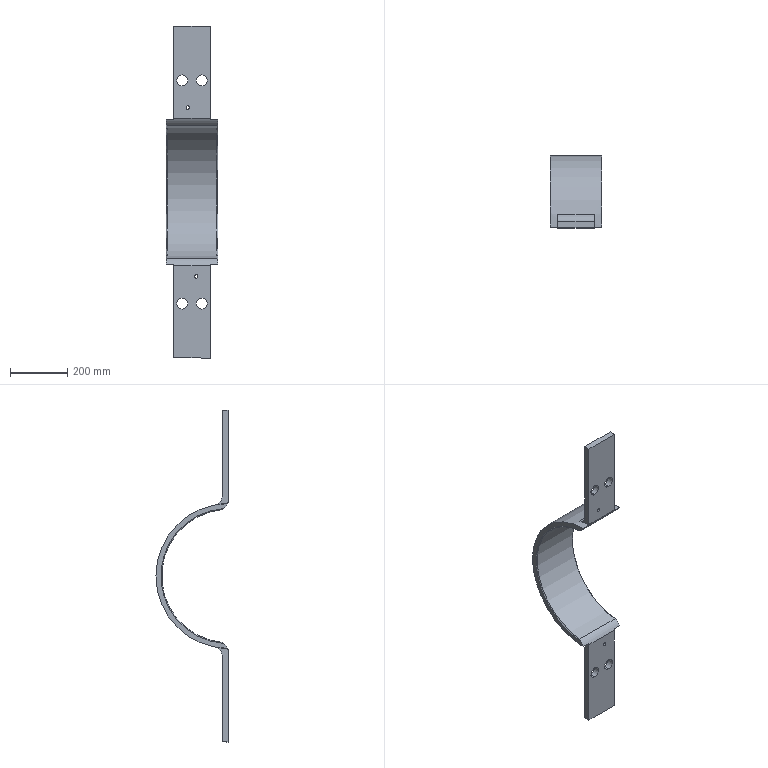Part | SolidWorks | features ICE 4, Fillet 2, MirrorPattern 2, Chamfer 1, Extrusion 1 | 1 solid | 32 faces | box 180 x 251.8 x 1160 mm | volume 4313938 mm3 | cylinder 18 | plane 12 | cone 2 | commonest cylinder face diameters 38 x8 12 x4 60 x2 110 x2 466 x1 506 x1
STEP:
#1=CARTESIAN_POINT('',(15.,22.,-301.));
#2=VERTEX_POINT('',#1);
#3=CARTESIAN_POINT('',(15.,22.,-289.));
#4=VERTEX_POINT('',#3);
#5=CARTESIAN_POINT('',(15.,22.,-295.));
#6=DIRECTION('',(0.,1.,0.));
#7=DIRECTION('',(0.,0.,-1.));
#8=AXIS2_PLACEMENT_3D('',#5,#6,#7);
#9=CIRCLE('',#8,6.);
#10=EDGE_CURVE('',#2,#4,#9,.T.);
#11=ORIENTED_EDGE('',*,*,#10,.T.);
#12=CARTESIAN_POINT('',(15.,1.2,-289.));
#13=VERTEX_POINT('',#12);
#14=CARTESIAN_POINT('',(15.,1.2,-289.));
#15=DIRECTION('',(0.,-1.,0.));
#16=VECTOR('',#15,1000.);
#17=LINE('',#14,#16);
#18=EDGE_CURVE('',#4,#13,#17,.T.);
#19=ORIENTED_EDGE('',*,*,#18,.T.);
#20=CARTESIAN_POINT('',(15.,1.2,-301.));
#21=VERTEX_POINT('',#20);
#22=CARTESIAN_POINT('',(15.,1.2,-295.));
#23=DIRECTION('',(0.,-1.,0.));
#24=DIRECTION('',(0.,0.,1.));
#25=AXIS2_PLACEMENT_3D('',#22,#23,#24);
#26=CIRCLE('',#25,6.);
#27=EDGE_CURVE('',#13,#21,#26,.T.);
#28=ORIENTED_EDGE('',*,*,#27,.T.);
#29=CARTESIAN_POINT('',(15.,1.2,-301.));
#30=DIRECTION('',(0.,-1.,0.));
#31=VECTOR('',#30,1000.);
#32=LINE('',#29,#31);
#33=EDGE_CURVE('',#2,#21,#32,.T.);
#34=ORIENTED_EDGE('',*,*,#33,.F.);
#35=EDGE_LOOP('',(#11,#19,#28,#34));
#36=FACE_OUTER_BOUND('',#35,.T.);
#37=CARTESIAN_POINT('',(15.,1.2,-295.));
#38=DIRECTION('',(0.,-1.,0.));
#39=DIRECTION('',(0.,0.,-1.));
#40=AXIS2_PLACEMENT_3D('',#37,#38,#39);
#41=CYLINDRICAL_SURFACE('',#40,6.);
#42=ADVANCED_FACE('',(#36),#41,.F.);
#43=CARTESIAN_POINT('',(-15.,22.,289.));
#44=VERTEX_POINT('',#43);
#45=CARTESIAN_POINT('',(-15.,22.,301.));
#46=VERTEX_POINT('',#45);
#47=CARTESIAN_POINT('',(-15.,22.,295.));
#48=DIRECTION('',(0.,1.,0.));
#49=DIRECTION('',(0.,0.,-1.));
#50=AXIS2_PLACEMENT_3D('',#47,#48,#49);
#51=CIRCLE('',#50,6.);
#52=EDGE_CURVE('',#44,#46,#51,.T.);
#53=ORIENTED_EDGE('',*,*,#52,.T.);
#54=CARTESIAN_POINT('',(-15.,1.2,301.));
#55=VERTEX_POINT('',#54);
#56=CARTESIAN_POINT('',(-15.,1.2,301.));
#57=DIRECTION('',(0.,-1.,0.));
#58=VECTOR('',#57,1000.);
#59=LINE('',#56,#58);
#60=EDGE_CURVE('',#46,#55,#59,.T.);
#61=ORIENTED_EDGE('',*,*,#60,.T.);
#62=CARTESIAN_POINT('',(-15.,1.2,289.));
#63=VERTEX_POINT('',#62);
#64=CARTESIAN_POINT('',(-15.,1.2,295.));
#65=DIRECTION('',(0.,-1.,0.));
#66=DIRECTION('',(0.,0.,1.));
#67=AXIS2_PLACEMENT_3D('',#64,#65,#66);
#68=CIRCLE('',#67,6.);
#69=EDGE_CURVE('',#55,#63,#68,.T.);
#70=ORIENTED_EDGE('',*,*,#69,.T.);
#71=CARTESIAN_POINT('',(-15.,1.2,289.));
#72=DIRECTION('',(0.,-1.,0.));
#73=VECTOR('',#72,1000.);
#74=LINE('',#71,#73);
#75=EDGE_CURVE('',#44,#63,#74,.T.);
#76=ORIENTED_EDGE('',*,*,#75,.F.);
#77=EDGE_LOOP('',(#53,#61,#70,#76));
#78=FACE_OUTER_BOUND('',#77,.T.);
#79=CARTESIAN_POINT('',(-15.,1.2,295.));
#80=DIRECTION('',(0.,-1.,0.));
#81=DIRECTION('',(0.,0.,-1.));
#82=AXIS2_PLACEMENT_3D('',#79,#80,#81);
#83=CYLINDRICAL_SURFACE('',#82,6.);
#84=ADVANCED_FACE('',(#78),#83,.F.);
#85=CARTESIAN_POINT('',(-34.,22.,-409.));
#86=VERTEX_POINT('',#85);
#87=CARTESIAN_POINT('',(-34.,22.,-371.));
#88=VERTEX_POINT('',#87);
#89=CARTESIAN_POINT('',(-34.,22.,-390.));
#90=DIRECTION('',(0.,1.,0.));
#91=DIRECTION('',(0.,0.,-1.));
#92=AXIS2_PLACEMENT_3D('',#89,#90,#91);
#93=CIRCLE('',#92,19.);
#94=EDGE_CURVE('',#86,#88,#93,.T.);
#95=ORIENTED_EDGE('',*,*,#94,.T.);
#96=CARTESIAN_POINT('',(-34.,1.2,-371.));
#97=VERTEX_POINT('',#96);
#98=CARTESIAN_POINT('',(-34.,1.2,-371.));
#99=DIRECTION('',(0.,-1.,0.));
#100=VECTOR('',#99,1000.);
#101=LINE('',#98,#100);
#102=EDGE_CURVE('',#88,#97,#101,.T.);
#103=ORIENTED_EDGE('',*,*,#102,.T.);
#104=CARTESIAN_POINT('',(-34.,1.2,-409.));
#105=VERTEX_POINT('',#104);
#106=CARTESIAN_POINT('',(-34.,1.2,-390.));
#107=DIRECTION('',(0.,-1.,0.));
#108=DIRECTION('',(0.,0.,1.));
#109=AXIS2_PLACEMENT_3D('',#106,#107,#108);
#110=CIRCLE('',#109,19.);
#111=EDGE_CURVE('',#97,#105,#110,.T.);
#112=ORIENTED_EDGE('',*,*,#111,.T.);
#113=CARTESIAN_POINT('',(-34.,1.2,-409.));
#114=DIRECTION('',(0.,-1.,0.));
#115=VECTOR('',#114,1000.);
#116=LINE('',#113,#115);
#117=EDGE_CURVE('',#86,#105,#116,.T.);
#118=ORIENTED_EDGE('',*,*,#117,.F.);
#119=EDGE_LOOP('',(#95,#103,#112,#118));
#120=FACE_OUTER_BOUND('',#119,.T.);
#121=CARTESIAN_POINT('',(-34.,1.2,-390.));
#122=DIRECTION('',(0.,-1.,0.));
#123=DIRECTION('',(0.,0.,-1.));
#124=AXIS2_PLACEMENT_3D('',#121,#122,#123);
#125=CYLINDRICAL_SURFACE('',#124,19.);
#126=ADVANCED_FACE('',(#120),#125,.F.);
#127=CARTESIAN_POINT('',(-34.,22.,371.));
#128=VERTEX_POINT('',#127);
#129=CARTESIAN_POINT('',(-34.,22.,409.));
#130=VERTEX_POINT('',#129);
#131=CARTESIAN_POINT('',(-34.,22.,390.));
#132=DIRECTION('',(0.,1.,0.));
#133=DIRECTION('',(0.,0.,-1.));
#134=AXIS2_PLACEMENT_3D('',#131,#132,#133);
#135=CIRCLE('',#134,19.);
#136=EDGE_CURVE('',#128,#130,#135,.T.);
#137=ORIENTED_EDGE('',*,*,#136,.T.);
#138=CARTESIAN_POINT('',(-34.,1.2,409.));
#139=VERTEX_POINT('',#138);
#140=CARTESIAN_POINT('',(-34.,1.2,409.));
#141=DIRECTION('',(0.,-1.,0.));
#142=VECTOR('',#141,1000.);
#143=LINE('',#140,#142);
#144=EDGE_CURVE('',#130,#139,#143,.T.);
#145=ORIENTED_EDGE('',*,*,#144,.T.);
#146=CARTESIAN_POINT('',(-34.,1.2,371.));
#147=VERTEX_POINT('',#146);
#148=CARTESIAN_POINT('',(-34.,1.2,390.));
#149=DIRECTION('',(0.,-1.,0.));
#150=DIRECTION('',(0.,0.,1.));
#151=AXIS2_PLACEMENT_3D('',#148,#149,#150);
#152=CIRCLE('',#151,19.);
#153=EDGE_CURVE('',#139,#147,#152,.T.);
#154=ORIENTED_EDGE('',*,*,#153,.T.);
#155=CARTESIAN_POINT('',(-34.,1.2,371.));
#156=DIRECTION('',(0.,-1.,0.));
#157=VECTOR('',#156,1000.);
#158=LINE('',#155,#157);
#159=EDGE_CURVE('',#128,#147,#158,.T.);
#160=ORIENTED_EDGE('',*,*,#159,.F.);
#161=EDGE_LOOP('',(#137,#145,#154,#160));
#162=FACE_OUTER_BOUND('',#161,.T.);
#163=CARTESIAN_POINT('',(-34.,1.2,390.));
#164=DIRECTION('',(0.,-1.,0.));
#165=DIRECTION('',(0.,0.,-1.));
#166=AXIS2_PLACEMENT_3D('',#163,#164,#165);
#167=CYLINDRICAL_SURFACE('',#166,19.);
#168=ADVANCED_FACE('',(#162),#167,.F.);
#169=CARTESIAN_POINT('',(34.,22.,-409.));
#170=VERTEX_POINT('',#169);
#171=CARTESIAN_POINT('',(34.,22.,-371.));
#172=VERTEX_POINT('',#171);
#173=CARTESIAN_POINT('',(34.,22.,-390.));
#174=DIRECTION('',(0.,1.,0.));
#175=DIRECTION('',(0.,0.,-1.));
#176=AXIS2_PLACEMENT_3D('',#173,#174,#175);
#177=CIRCLE('',#176,19.);
#178=EDGE_CURVE('',#170,#172,#177,.T.);
#179=ORIENTED_EDGE('',*,*,#178,.T.);
#180=CARTESIAN_POINT('',(34.,1.2,-371.));
#181=VERTEX_POINT('',#180);
#182=CARTESIAN_POINT('',(34.,1.2,-371.));
#183=DIRECTION('',(0.,-1.,0.));
#184=VECTOR('',#183,1000.);
#185=LINE('',#182,#184);
#186=EDGE_CURVE('',#172,#181,#185,.T.);
#187=ORIENTED_EDGE('',*,*,#186,.T.);
#188=CARTESIAN_POINT('',(34.,1.2,-409.));
#189=VERTEX_POINT('',#188);
#190=CARTESIAN_POINT('',(34.,1.2,-390.));
#191=DIRECTION('',(0.,-1.,0.));
#192=DIRECTION('',(0.,0.,1.));
#193=AXIS2_PLACEMENT_3D('',#190,#191,#192);
#194=CIRCLE('',#193,19.);
#195=EDGE_CURVE('',#181,#189,#194,.T.);
#196=ORIENTED_EDGE('',*,*,#195,.T.);
#197=CARTESIAN_POINT('',(34.,1.2,-409.));
#198=DIRECTION('',(0.,-1.,0.));
#199=VECTOR('',#198,1000.);
#200=LINE('',#197,#199);
#201=EDGE_CURVE('',#170,#189,#200,.T.);
#202=ORIENTED_EDGE('',*,*,#201,.F.);
#203=EDGE_LOOP('',(#179,#187,#196,#202));
#204=FACE_OUTER_BOUND('',#203,.T.);
#205=CARTESIAN_POINT('',(34.,1.2,-390.));
#206=DIRECTION('',(0.,-1.,0.));
#207=DIRECTION('',(0.,0.,-1.));
#208=AXIS2_PLACEMENT_3D('',#205,#206,#207);
#209=CYLINDRICAL_SURFACE('',#208,19.);
#210=ADVANCED_FACE('',(#204),#209,.F.);
#211=CARTESIAN_POINT('',(34.,22.,371.));
#212=VERTEX_POINT('',#211);
#213=CARTESIAN_POINT('',(34.,22.,409.));
#214=VERTEX_POINT('',#213);
#215=CARTESIAN_POINT('',(34.,22.,390.));
#216=DIRECTION('',(0.,1.,0.));
#217=DIRECTION('',(0.,0.,-1.));
#218=AXIS2_PLACEMENT_3D('',#215,#216,#217);
#219=CIRCLE('',#218,19.);
#220=EDGE_CURVE('',#212,#214,#219,.T.);
#221=ORIENTED_EDGE('',*,*,#220,.T.);
#222=CARTESIAN_POINT('',(34.,1.2,409.));
#223=VERTEX_POINT('',#222);
#224=CARTESIAN_POINT('',(34.,1.2,409.));
#225=DIRECTION('',(0.,-1.,0.));
#226=VECTOR('',#225,1000.);
#227=LINE('',#224,#226);
#228=EDGE_CURVE('',#214,#223,#227,.T.);
#229=ORIENTED_EDGE('',*,*,#228,.T.);
#230=CARTESIAN_POINT('',(34.,1.2,371.));
#231=VERTEX_POINT('',#230);
#232=CARTESIAN_POINT('',(34.,1.2,390.));
#233=DIRECTION('',(0.,-1.,0.));
#234=DIRECTION('',(0.,0.,1.));
#235=AXIS2_PLACEMENT_3D('',#232,#233,#234);
#236=CIRCLE('',#235,19.);
#237=EDGE_CURVE('',#223,#231,#236,.T.);
#238=ORIENTED_EDGE('',*,*,#237,.T.);
#239=CARTESIAN_POINT('',(34.,1.2,371.));
#240=DIRECTION('',(0.,-1.,0.));
#241=VECTOR('',#240,1000.);
#242=LINE('',#239,#241);
#243=EDGE_CURVE('',#212,#231,#242,.T.);
#244=ORIENTED_EDGE('',*,*,#243,.F.);
#245=EDGE_LOOP('',(#221,#229,#238,#244));
#246=FACE_OUTER_BOUND('',#245,.T.);
#247=CARTESIAN_POINT('',(34.,1.2,390.));
#248=DIRECTION('',(0.,-1.,0.));
#249=DIRECTION('',(0.,0.,-1.));
#250=AXIS2_PLACEMENT_3D('',#247,#248,#249);
#251=CYLINDRICAL_SURFACE('',#250,19.);
#252=ADVANCED_FACE('',(#246),#251,.F.);
#253=ORIENTED_EDGE('',*,*,#94,.F.);
#254=CARTESIAN_POINT('',(-34.,22.,-390.));
#255=DIRECTION('',(0.,1.,0.));
#256=DIRECTION('',(0.,0.,-1.));
#257=AXIS2_PLACEMENT_3D('',#254,#255,#256);
#258=CIRCLE('',#257,19.);
#259=EDGE_CURVE('',#88,#86,#258,.T.);
#260=ORIENTED_EDGE('',*,*,#259,.F.);
#261=EDGE_LOOP('',(#253,#260));
#262=FACE_BOUND('',#261,.T.);
#263=CARTESIAN_POINT('',(-63.,22.,-278.182));
#264=VERTEX_POINT('',#263);
#265=CARTESIAN_POINT('',(-63.,22.,-580.));
#266=VERTEX_POINT('',#265);
#267=CARTESIAN_POINT('',(-63.,22.,-252.042));
#268=DIRECTION('',(0.,0.,-1.));
#269=VECTOR('',#268,1000.);
#270=LINE('',#267,#269);
#271=EDGE_CURVE('',#264,#266,#270,.T.);
#272=ORIENTED_EDGE('',*,*,#271,.F.);
#273=CARTESIAN_POINT('',(63.,22.,-278.182));
#274=VERTEX_POINT('',#273);
#275=CARTESIAN_POINT('',(90.,22.,-278.182));
#276=DIRECTION('',(1.,0.,0.));
#277=VECTOR('',#276,1000.);
#278=LINE('',#275,#277);
#279=EDGE_CURVE('',#264,#274,#278,.T.);
#280=ORIENTED_EDGE('',*,*,#279,.T.);
#281=CARTESIAN_POINT('',(63.,22.,-580.));
#282=VERTEX_POINT('',#281);
#283=CARTESIAN_POINT('',(63.,22.,-252.042));
#284=DIRECTION('',(0.,0.,1.));
#285=VECTOR('',#284,1000.);
#286=LINE('',#283,#285);
#287=EDGE_CURVE('',#282,#274,#286,.T.);
#288=ORIENTED_EDGE('',*,*,#287,.F.);
#289=CARTESIAN_POINT('',(90.,22.,-580.));
#290=DIRECTION('',(-1.,0.,0.));
#291=VECTOR('',#290,1000.);
#292=LINE('',#289,#291);
#293=EDGE_CURVE('',#282,#266,#292,.T.);
#294=ORIENTED_EDGE('',*,*,#293,.T.);
#295=EDGE_LOOP('',(#272,#280,#288,#294));
#296=FACE_OUTER_BOUND('',#295,.T.);
#297=ORIENTED_EDGE('',*,*,#178,.F.);
#298=CARTESIAN_POINT('',(34.,22.,-390.));
#299=DIRECTION('',(0.,1.,0.));
#300=DIRECTION('',(0.,0.,-1.));
#301=AXIS2_PLACEMENT_3D('',#298,#299,#300);
#302=CIRCLE('',#301,19.);
#303=EDGE_CURVE('',#172,#170,#302,.T.);
#304=ORIENTED_EDGE('',*,*,#303,.F.);
#305=EDGE_LOOP('',(#297,#304));
#306=FACE_BOUND('',#305,.T.);
#307=ORIENTED_EDGE('',*,*,#10,.F.);
#308=CARTESIAN_POINT('',(15.,22.,-295.));
#309=DIRECTION('',(0.,1.,0.));
#310=DIRECTION('',(0.,0.,-1.));
#311=AXIS2_PLACEMENT_3D('',#308,#309,#310);
#312=CIRCLE('',#311,6.);
#313=EDGE_CURVE('',#4,#2,#312,.T.);
#314=ORIENTED_EDGE('',*,*,#313,.F.);
#315=EDGE_LOOP('',(#307,#314));
#316=FACE_BOUND('',#315,.T.);
#317=CARTESIAN_POINT('',(90.,22.,-252.042));
#318=DIRECTION('',(0.,-1.,0.));
#319=DIRECTION('',(0.,0.,-1.));
#320=AXIS2_PLACEMENT_3D('',#317,#318,#319);
#321=PLANE('',#320);
#322=ADVANCED_FACE('',(#262,#296,#306,#316),#321,.F.);
#323=CARTESIAN_POINT('',(-34.,1.2,-390.));
#324=DIRECTION('',(0.,-1.,0.));
#325=DIRECTION('',(0.,0.,1.));
#326=AXIS2_PLACEMENT_3D('',#323,#324,#325);
#327=CIRCLE('',#326,19.);
#328=EDGE_CURVE('',#105,#97,#327,.T.);
#329=ORIENTED_EDGE('',*,*,#328,.F.);
#330=ORIENTED_EDGE('',*,*,#111,.F.);
#331=EDGE_LOOP('',(#329,#330));
#332=FACE_BOUND('',#331,.T.);
#333=CARTESIAN_POINT('',(-63.,1.2,-580.));
#334=VERTEX_POINT('',#333);
#335=CARTESIAN_POINT('',(-63.,1.2,-257.102));
#336=VERTEX_POINT('',#335);
#337=CARTESIAN_POINT('',(-63.,1.2,610.));
#338=DIRECTION('',(0.,0.,1.));
#339=VECTOR('',#338,1000.);
#340=LINE('',#337,#339);
#341=EDGE_CURVE('',#334,#336,#340,.T.);
#342=ORIENTED_EDGE('',*,*,#341,.F.);
#343=CARTESIAN_POINT('',(63.,1.2,-580.));
#344=VERTEX_POINT('',#343);
#345=CARTESIAN_POINT('',(90.,1.2,-580.));
#346=DIRECTION('',(-1.,0.,0.));
#347=VECTOR('',#346,1000.);
#348=LINE('',#345,#347);
#349=EDGE_CURVE('',#344,#334,#348,.T.);
#350=ORIENTED_EDGE('',*,*,#349,.F.);
#351=CARTESIAN_POINT('',(63.,1.2,-257.102));
#352=VERTEX_POINT('',#351);
#353=CARTESIAN_POINT('',(63.,1.2,610.));
#354=DIRECTION('',(0.,0.,-1.));
#355=VECTOR('',#354,1000.);
#356=LINE('',#353,#355);
#357=EDGE_CURVE('',#352,#344,#356,.T.);
#358=ORIENTED_EDGE('',*,*,#357,.F.);
#359=CARTESIAN_POINT('',(90.,1.2,-257.102));
#360=DIRECTION('',(-1.,0.,0.));
#361=VECTOR('',#360,1000.);
#362=LINE('',#359,#361);
#363=EDGE_CURVE('',#352,#336,#362,.T.);
#364=ORIENTED_EDGE('',*,*,#363,.T.);
#365=EDGE_LOOP('',(#342,#350,#358,#364));
#366=FACE_OUTER_BOUND('',#365,.T.);
#367=CARTESIAN_POINT('',(34.,1.2,-390.));
#368=DIRECTION('',(0.,-1.,0.));
#369=DIRECTION('',(0.,0.,1.));
#370=AXIS2_PLACEMENT_3D('',#367,#368,#369);
#371=CIRCLE('',#370,19.);
#372=EDGE_CURVE('',#189,#181,#371,.T.);
#373=ORIENTED_EDGE('',*,*,#372,.F.);
#374=ORIENTED_EDGE('',*,*,#195,.F.);
#375=EDGE_LOOP('',(#373,#374));
#376=FACE_BOUND('',#375,.T.);
#377=CARTESIAN_POINT('',(15.,1.2,-295.));
#378=DIRECTION('',(0.,-1.,0.));
#379=DIRECTION('',(0.,0.,1.));
#380=AXIS2_PLACEMENT_3D('',#377,#378,#379);
#381=CIRCLE('',#380,6.);
#382=EDGE_CURVE('',#21,#13,#381,.T.);
#383=ORIENTED_EDGE('',*,*,#382,.F.);
#384=ORIENTED_EDGE('',*,*,#27,.F.);
#385=EDGE_LOOP('',(#383,#384));
#386=FACE_BOUND('',#385,.T.);
#387=CARTESIAN_POINT('',(-90.,1.2,610.));
#388=DIRECTION('',(0.,1.,0.));
#389=DIRECTION('',(0.,0.,1.));
#390=AXIS2_PLACEMENT_3D('',#387,#388,#389);
#391=PLANE('',#390);
#392=ADVANCED_FACE('',(#332,#366,#376,#386),#391,.F.);
#393=ORIENTED_EDGE('',*,*,#136,.F.);
#394=CARTESIAN_POINT('',(-34.,22.,390.));
#395=DIRECTION('',(0.,1.,0.));
#396=DIRECTION('',(0.,0.,-1.));
#397=AXIS2_PLACEMENT_3D('',#394,#395,#396);
#398=CIRCLE('',#397,19.);
#399=EDGE_CURVE('',#130,#128,#398,.T.);
#400=ORIENTED_EDGE('',*,*,#399,.F.);
#401=EDGE_LOOP('',(#393,#400));
#402=FACE_BOUND('',#401,.T.);
#403=CARTESIAN_POINT('',(-63.,22.,580.));
#404=VERTEX_POINT('',#403);
#405=CARTESIAN_POINT('',(-63.,22.,278.182));
#406=VERTEX_POINT('',#405);
#407=CARTESIAN_POINT('',(-63.,22.,580.));
#408=DIRECTION('',(0.,0.,-1.));
#409=VECTOR('',#408,1000.);
#410=LINE('',#407,#409);
#411=EDGE_CURVE('',#404,#406,#410,.T.);
#412=ORIENTED_EDGE('',*,*,#411,.F.);
#413=CARTESIAN_POINT('',(63.,22.,580.));
#414=VERTEX_POINT('',#413);
#415=CARTESIAN_POINT('',(90.,22.,580.));
#416=DIRECTION('',(-1.,0.,0.));
#417=VECTOR('',#416,1000.);
#418=LINE('',#415,#417);
#419=EDGE_CURVE('',#414,#404,#418,.T.);
#420=ORIENTED_EDGE('',*,*,#419,.F.);
#421=CARTESIAN_POINT('',(63.,22.,278.182));
#422=VERTEX_POINT('',#421);
#423=CARTESIAN_POINT('',(63.,22.,580.));
#424=DIRECTION('',(0.,0.,1.));
#425=VECTOR('',#424,1000.);
#426=LINE('',#423,#425);
#427=EDGE_CURVE('',#422,#414,#426,.T.);
#428=ORIENTED_EDGE('',*,*,#427,.F.);
#429=CARTESIAN_POINT('',(-90.,22.,278.182));
#430=DIRECTION('',(-1.,0.,0.));
#431=VECTOR('',#430,1000.);
#432=LINE('',#429,#431);
#433=EDGE_CURVE('',#422,#406,#432,.T.);
#434=ORIENTED_EDGE('',*,*,#433,.T.);
#435=EDGE_LOOP('',(#412,#420,#428,#434));
#436=FACE_OUTER_BOUND('',#435,.T.);
#437=ORIENTED_EDGE('',*,*,#220,.F.);
#438=CARTESIAN_POINT('',(34.,22.,390.));
#439=DIRECTION('',(0.,1.,0.));
#440=DIRECTION('',(0.,0.,-1.));
#441=AXIS2_PLACEMENT_3D('',#438,#439,#440);
#442=CIRCLE('',#441,19.);
#443=EDGE_CURVE('',#214,#212,#442,.T.);
#444=ORIENTED_EDGE('',*,*,#443,.F.);
#445=EDGE_LOOP('',(#437,#444));
#446=FACE_BOUND('',#445,.T.);
#447=ORIENTED_EDGE('',*,*,#52,.F.);
#448=CARTESIAN_POINT('',(-15.,22.,295.));
#449=DIRECTION('',(0.,1.,0.));
#450=DIRECTION('',(0.,0.,-1.));
#451=AXIS2_PLACEMENT_3D('',#448,#449,#450);
#452=CIRCLE('',#451,6.);
#453=EDGE_CURVE('',#46,#44,#452,.T.);
#454=ORIENTED_EDGE('',*,*,#453,.F.);
#455=EDGE_LOOP('',(#447,#454));
#456=FACE_BOUND('',#455,.T.);
#457=CARTESIAN_POINT('',(90.,22.,580.));
#458=DIRECTION('',(0.,-1.,0.));
#459=DIRECTION('',(0.,0.,-1.));
#460=AXIS2_PLACEMENT_3D('',#457,#458,#459);
#461=PLANE('',#460);
#462=ADVANCED_FACE('',(#402,#436,#446,#456),#461,.F.);
#463=CARTESIAN_POINT('',(-34.,1.2,390.));
#464=DIRECTION('',(0.,-1.,0.));
#465=DIRECTION('',(0.,0.,1.));
#466=AXIS2_PLACEMENT_3D('',#463,#464,#465);
#467=CIRCLE('',#466,19.);
#468=EDGE_CURVE('',#147,#139,#467,.T.);
#469=ORIENTED_EDGE('',*,*,#468,.F.);
#470=ORIENTED_EDGE('',*,*,#153,.F.);
#471=EDGE_LOOP('',(#469,#470));
#472=FACE_BOUND('',#471,.T.);
#473=CARTESIAN_POINT('',(-63.,1.2,257.102));
#474=VERTEX_POINT('',#473);
#475=CARTESIAN_POINT('',(-63.,1.2,580.));
#476=VERTEX_POINT('',#475);
#477=CARTESIAN_POINT('',(-63.,1.2,610.));
#478=DIRECTION('',(0.,0.,1.));
#479=VECTOR('',#478,1000.);
#480=LINE('',#477,#479);
#481=EDGE_CURVE('',#474,#476,#480,.T.);
#482=ORIENTED_EDGE('',*,*,#481,.F.);
#483=CARTESIAN_POINT('',(63.,1.2,257.102));
#484=VERTEX_POINT('',#483);
#485=CARTESIAN_POINT('',(90.,1.2,257.102));
#486=DIRECTION('',(1.,0.,0.));
#487=VECTOR('',#486,1000.);
#488=LINE('',#485,#487);
#489=EDGE_CURVE('',#474,#484,#488,.T.);
#490=ORIENTED_EDGE('',*,*,#489,.T.);
#491=CARTESIAN_POINT('',(63.,1.2,580.));
#492=VERTEX_POINT('',#491);
#493=CARTESIAN_POINT('',(63.,1.2,610.));
#494=DIRECTION('',(0.,0.,-1.));
#495=VECTOR('',#494,1000.);
#496=LINE('',#493,#495);
#497=EDGE_CURVE('',#492,#484,#496,.T.);
#498=ORIENTED_EDGE('',*,*,#497,.F.);
#499=CARTESIAN_POINT('',(90.,1.2,580.));
#500=DIRECTION('',(1.,0.,0.));
#501=VECTOR('',#500,1000.);
#502=LINE('',#499,#501);
#503=EDGE_CURVE('',#476,#492,#502,.T.);
#504=ORIENTED_EDGE('',*,*,#503,.F.);
#505=EDGE_LOOP('',(#482,#490,#498,#504));
#506=FACE_OUTER_BOUND('',#505,.T.);
#507=CARTESIAN_POINT('',(34.,1.2,390.));
#508=DIRECTION('',(0.,-1.,0.));
#509=DIRECTION('',(0.,0.,1.));
#510=AXIS2_PLACEMENT_3D('',#507,#508,#509);
#511=CIRCLE('',#510,19.);
#512=EDGE_CURVE('',#231,#223,#511,.T.);
#513=ORIENTED_EDGE('',*,*,#512,.F.);
#514=ORIENTED_EDGE('',*,*,#237,.F.);
#515=EDGE_LOOP('',(#513,#514));
#516=FACE_BOUND('',#515,.T.);
#517=CARTESIAN_POINT('',(-15.,1.2,295.));
#518=DIRECTION('',(0.,-1.,0.));
#519=DIRECTION('',(0.,0.,1.));
#520=AXIS2_PLACEMENT_3D('',#517,#518,#519);
#521=CIRCLE('',#520,6.);
#522=EDGE_CURVE('',#63,#55,#521,.T.);
#523=ORIENTED_EDGE('',*,*,#522,.F.);
#524=ORIENTED_EDGE('',*,*,#69,.F.);
#525=EDGE_LOOP('',(#523,#524));
#526=FACE_BOUND('',#525,.T.);
#527=CARTESIAN_POINT('',(-90.,1.2,610.));
#528=DIRECTION('',(0.,1.,0.));
#529=DIRECTION('',(0.,0.,1.));
#530=AXIS2_PLACEMENT_3D('',#527,#528,#529);
#531=PLANE('',#530);
#532=ADVANCED_FACE('',(#472,#506,#516,#526),#531,.F.);
#533=CARTESIAN_POINT('',(-63.,22.,-580.));
#534=DIRECTION('',(0.,-1.,0.));
#535=VECTOR('',#534,1000.);
#536=LINE('',#533,#535);
#537=EDGE_CURVE('',#266,#334,#536,.T.);
#538=ORIENTED_EDGE('',*,*,#537,.F.);
#539=ORIENTED_EDGE('',*,*,#293,.F.);
#540=CARTESIAN_POINT('',(63.,22.,-580.));
#541=DIRECTION('',(0.,1.,0.));
#542=VECTOR('',#541,1000.);
#543=LINE('',#540,#542);
#544=EDGE_CURVE('',#344,#282,#543,.T.);
#545=ORIENTED_EDGE('',*,*,#544,.F.);
#546=ORIENTED_EDGE('',*,*,#349,.T.);
#547=EDGE_LOOP('',(#538,#539,#545,#546));
#548=FACE_OUTER_BOUND('',#547,.T.);
#549=CARTESIAN_POINT('',(90.,22.,-580.));
#550=DIRECTION('',(0.,0.,1.));
#551=DIRECTION('',(1.,0.,0.));
#552=AXIS2_PLACEMENT_3D('',#549,#550,#551);
#553=PLANE('',#552);
#554=ADVANCED_FACE('',(#548),#553,.F.);
#555=CARTESIAN_POINT('',(-63.,46.488,-248.692));
#556=VERTEX_POINT('',#555);
#557=CARTESIAN_POINT('',(-63.,52.,-278.182));
#558=DIRECTION('',(1.,0.,0.));
#559=DIRECTION('',(0.,0.,1.));
#560=AXIS2_PLACEMENT_3D('',#557,#558,#559);
#561=CIRCLE('',#560,30.);
#562=EDGE_CURVE('',#556,#264,#561,.T.);
#563=ORIENTED_EDGE('',*,*,#562,.F.);
#564=CARTESIAN_POINT('',(63.,46.488,-248.692));
#565=VERTEX_POINT('',#564);
#566=CARTESIAN_POINT('',(90.,46.488,-248.692));
#567=DIRECTION('',(-1.,0.,0.));
#568=VECTOR('',#567,1000.);
#569=LINE('',#566,#568);
#570=EDGE_CURVE('',#565,#556,#569,.T.);
#571=ORIENTED_EDGE('',*,*,#570,.F.);
#572=CARTESIAN_POINT('',(63.,52.,-278.182));
#573=DIRECTION('',(-1.,0.,0.));
#574=DIRECTION('',(0.,0.,-1.));
#575=AXIS2_PLACEMENT_3D('',#572,#573,#574);
#576=CIRCLE('',#575,30.);
#577=EDGE_CURVE('',#274,#565,#576,.T.);
#578=ORIENTED_EDGE('',*,*,#577,.F.);
#579=ORIENTED_EDGE('',*,*,#279,.F.);
#580=EDGE_LOOP('',(#563,#571,#578,#579));
#581=FACE_OUTER_BOUND('',#580,.T.);
#582=CARTESIAN_POINT('',(90.,52.,-278.182));
#583=DIRECTION('',(-1.,0.,0.));
#584=DIRECTION('',(0.,0.,1.));
#585=AXIS2_PLACEMENT_3D('',#582,#583,#584);
#586=CYLINDRICAL_SURFACE('',#585,30.);
#587=ADVANCED_FACE('',(#581),#586,.F.);
#588=CARTESIAN_POINT('',(-63.,22.,580.));
#589=DIRECTION('',(0.,1.,0.));
#590=VECTOR('',#589,1000.);
#591=LINE('',#588,#590);
#592=EDGE_CURVE('',#476,#404,#591,.T.);
#593=ORIENTED_EDGE('',*,*,#592,.F.);
#594=ORIENTED_EDGE('',*,*,#503,.T.);
#595=CARTESIAN_POINT('',(63.,22.,580.));
#596=DIRECTION('',(0.,-1.,0.));
#597=VECTOR('',#596,1000.);
#598=LINE('',#595,#597);
#599=EDGE_CURVE('',#414,#492,#598,.T.);
#600=ORIENTED_EDGE('',*,*,#599,.F.);
#601=ORIENTED_EDGE('',*,*,#419,.T.);
#602=EDGE_LOOP('',(#593,#594,#600,#601));
#603=FACE_OUTER_BOUND('',#602,.T.);
#604=CARTESIAN_POINT('',(90.,22.,580.));
#605=DIRECTION('',(0.,0.,-1.));
#606=DIRECTION('',(-1.,0.,0.));
#607=AXIS2_PLACEMENT_3D('',#604,#605,#606);
#608=PLANE('',#607);
#609=ADVANCED_FACE('',(#603),#608,.F.);
#610=CARTESIAN_POINT('',(-63.,46.488,248.692));
#611=VERTEX_POINT('',#610);
#612=CARTESIAN_POINT('',(-63.,52.,278.182));
#613=DIRECTION('',(1.,0.,0.));
#614=DIRECTION('',(0.,0.,1.));
#615=AXIS2_PLACEMENT_3D('',#612,#613,#614);
#616=CIRCLE('',#615,30.);
#617=EDGE_CURVE('',#406,#611,#616,.T.);
#618=ORIENTED_EDGE('',*,*,#617,.F.);
#619=ORIENTED_EDGE('',*,*,#433,.F.);
#620=CARTESIAN_POINT('',(63.,46.488,248.692));
#621=VERTEX_POINT('',#620);
#622=CARTESIAN_POINT('',(63.,52.,278.182));
#623=DIRECTION('',(-1.,0.,0.));
#624=DIRECTION('',(0.,0.,-1.));
#625=AXIS2_PLACEMENT_3D('',#622,#623,#624);
#626=CIRCLE('',#625,30.);
#627=EDGE_CURVE('',#621,#422,#626,.T.);
#628=ORIENTED_EDGE('',*,*,#627,.F.);
#629=CARTESIAN_POINT('',(90.,46.488,248.692));
#630=DIRECTION('',(1.,0.,0.));
#631=VECTOR('',#630,1000.);
#632=LINE('',#629,#631);
#633=EDGE_CURVE('',#611,#621,#632,.T.);
#634=ORIENTED_EDGE('',*,*,#633,.F.);
#635=EDGE_LOOP('',(#618,#619,#628,#634));
#636=FACE_OUTER_BOUND('',#635,.T.);
#637=CARTESIAN_POINT('',(90.,52.,278.182));
#638=DIRECTION('',(-1.,0.,0.));
#639=DIRECTION('',(0.,0.,1.));
#640=AXIS2_PLACEMENT_3D('',#637,#638,#639);
#641=CYLINDRICAL_SURFACE('',#640,30.);
#642=ADVANCED_FACE('',(#636),#641,.F.);
#643=CARTESIAN_POINT('',(-90.,3.113,-252.981));
#644=VERTEX_POINT('',#643);
#645=CARTESIAN_POINT('',(-90.,17.496,-235.351));
#646=VERTEX_POINT('',#645);
#647=CARTESIAN_POINT('',(-90.,52.,-278.182));
#648=DIRECTION('',(-1.,0.,0.));
#649=DIRECTION('',(0.,0.,-1.));
#650=AXIS2_PLACEMENT_3D('',#647,#648,#649);
#651=CIRCLE('',#650,55.);
#652=EDGE_CURVE('',#644,#646,#651,.T.);
#653=ORIENTED_EDGE('',*,*,#652,.T.);
#654=CARTESIAN_POINT('',(-90.,17.496,235.351));
#655=VERTEX_POINT('',#654);
#656=CARTESIAN_POINT('',(-90.,0.,0.));
#657=DIRECTION('',(1.,0.,0.));
#658=DIRECTION('',(0.,0.,-1.));
#659=AXIS2_PLACEMENT_3D('',#656,#657,#658);
#660=CIRCLE('',#659,236.);
#661=EDGE_CURVE('',#646,#655,#660,.T.);
#662=ORIENTED_EDGE('',*,*,#661,.T.);
#663=CARTESIAN_POINT('',(-90.,3.113,252.981));
#664=VERTEX_POINT('',#663);
#665=CARTESIAN_POINT('',(-90.,52.,278.182));
#666=DIRECTION('',(-1.,0.,0.));
#667=DIRECTION('',(0.,0.,-1.));
#668=AXIS2_PLACEMENT_3D('',#665,#666,#667);
#669=CIRCLE('',#668,55.);
#670=EDGE_CURVE('',#655,#664,#669,.T.);
#671=ORIENTED_EDGE('',*,*,#670,.T.);
#672=CARTESIAN_POINT('',(-90.,0.,0.));
#673=DIRECTION('',(1.,0.,0.));
#674=DIRECTION('',(0.,0.,-1.));
#675=AXIS2_PLACEMENT_3D('',#672,#673,#674);
#676=CIRCLE('',#675,253.);
#677=EDGE_CURVE('',#644,#664,#676,.T.);
#678=ORIENTED_EDGE('',*,*,#677,.F.);
#679=EDGE_LOOP('',(#653,#662,#671,#678));
#680=FACE_OUTER_BOUND('',#679,.T.);
#681=CARTESIAN_POINT('',(-90.,0.,0.));
#682=DIRECTION('',(1.,0.,0.));
#683=DIRECTION('',(0.,0.,-1.));
#684=AXIS2_PLACEMENT_3D('',#681,#682,#683);
#685=PLANE('',#684);
#686=ADVANCED_FACE('',(#680),#685,.F.);
#687=ORIENTED_EDGE('',*,*,#670,.F.);
#688=CARTESIAN_POINT('',(-87.,22.226,231.937));
#689=VERTEX_POINT('',#688);
#690=CARTESIAN_POINT('',(-90.,17.496,235.351));
#691=CARTESIAN_POINT('',(-88.918,18.98,234.156));
#692=CARTESIAN_POINT('',(-87.913,20.552,233.016));
#693=CARTESIAN_POINT('',(-87.,22.226,231.937));
#694=B_SPLINE_CURVE_WITH_KNOTS('',3,(#690,#691,#692,#693),.UNSPECIFIED.,.F.,.F.,(4,4),(0.,0.006559),.UNSPECIFIED.);
#695=EDGE_CURVE('',#655,#689,#694,.T.);
#696=ORIENTED_EDGE('',*,*,#695,.T.);
#697=CARTESIAN_POINT('',(87.,22.226,231.937));
#698=VERTEX_POINT('',#697);
#699=CARTESIAN_POINT('',(0.,22.226,231.937));
#700=DIRECTION('',(-1.,0.,0.));
#701=VECTOR('',#700,1000.);
#702=LINE('',#699,#701);
#703=EDGE_CURVE('',#698,#689,#702,.T.);
#704=ORIENTED_EDGE('',*,*,#703,.F.);
#705=CARTESIAN_POINT('',(90.,17.496,235.351));
#706=VERTEX_POINT('',#705);
#707=CARTESIAN_POINT('',(87.,22.226,231.937));
#708=CARTESIAN_POINT('',(87.913,20.552,233.016));
#709=CARTESIAN_POINT('',(88.918,18.98,234.156));
#710=CARTESIAN_POINT('',(90.,17.496,235.351));
#711=B_SPLINE_CURVE_WITH_KNOTS('',3,(#707,#708,#709,#710),.UNSPECIFIED.,.F.,.F.,(4,4),(0.,0.006559),.UNSPECIFIED.);
#712=EDGE_CURVE('',#698,#706,#711,.T.);
#713=ORIENTED_EDGE('',*,*,#712,.T.);
#714=CARTESIAN_POINT('',(90.,3.113,252.981));
#715=VERTEX_POINT('',#714);
#716=CARTESIAN_POINT('',(90.,52.,278.182));
#717=DIRECTION('',(1.,0.,0.));
#718=DIRECTION('',(0.,0.,-1.));
#719=AXIS2_PLACEMENT_3D('',#716,#717,#718);
#720=CIRCLE('',#719,55.);
#721=EDGE_CURVE('',#715,#706,#720,.T.);
#722=ORIENTED_EDGE('',*,*,#721,.F.);
#723=CARTESIAN_POINT('',(63.,3.113,252.981));
#724=VERTEX_POINT('',#723);
#725=CARTESIAN_POINT('',(76.5,3.113,252.981));
#726=DIRECTION('',(1.,0.,0.));
#727=VECTOR('',#726,1000.);
#728=LINE('',#725,#727);
#729=EDGE_CURVE('',#724,#715,#728,.T.);
#730=ORIENTED_EDGE('',*,*,#729,.F.);
#731=CARTESIAN_POINT('',(63.,52.,278.182));
#732=DIRECTION('',(-1.,0.,0.));
#733=DIRECTION('',(0.,0.,-1.));
#734=AXIS2_PLACEMENT_3D('',#731,#732,#733);
#735=CIRCLE('',#734,55.);
#736=EDGE_CURVE('',#724,#484,#735,.T.);
#737=ORIENTED_EDGE('',*,*,#736,.T.);
#738=ORIENTED_EDGE('',*,*,#489,.F.);
#739=CARTESIAN_POINT('',(-63.,3.113,252.981));
#740=VERTEX_POINT('',#739);
#741=CARTESIAN_POINT('',(-63.,52.,278.182));
#742=DIRECTION('',(1.,0.,0.));
#743=DIRECTION('',(0.,0.,1.));
#744=AXIS2_PLACEMENT_3D('',#741,#742,#743);
#745=CIRCLE('',#744,55.);
#746=EDGE_CURVE('',#474,#740,#745,.T.);
#747=ORIENTED_EDGE('',*,*,#746,.T.);
#748=CARTESIAN_POINT('',(-76.5,3.113,252.981));
#749=DIRECTION('',(-1.,0.,0.));
#750=VECTOR('',#749,1000.);
#751=LINE('',#748,#750);
#752=EDGE_CURVE('',#740,#664,#751,.T.);
#753=ORIENTED_EDGE('',*,*,#752,.T.);
#754=EDGE_LOOP('',(#687,#696,#704,#713,#722,#730,#737,#738,#747,#753));
#755=FACE_OUTER_BOUND('',#754,.T.);
#756=CARTESIAN_POINT('',(90.,52.,278.182));
#757=DIRECTION('',(-1.,0.,0.));
#758=DIRECTION('',(0.,0.,1.));
#759=AXIS2_PLACEMENT_3D('',#756,#757,#758);
#760=CYLINDRICAL_SURFACE('',#759,55.);
#761=ADVANCED_FACE('',(#755),#760,.T.);
#762=ORIENTED_EDGE('',*,*,#721,.T.);
#763=CARTESIAN_POINT('',(90.,17.496,-235.351));
#764=VERTEX_POINT('',#763);
#765=CARTESIAN_POINT('',(90.,0.,0.));
#766=DIRECTION('',(-1.,0.,0.));
#767=DIRECTION('',(0.,0.,-1.));
#768=AXIS2_PLACEMENT_3D('',#765,#766,#767);
#769=CIRCLE('',#768,236.);
#770=EDGE_CURVE('',#706,#764,#769,.T.);
#771=ORIENTED_EDGE('',*,*,#770,.T.);
#772=CARTESIAN_POINT('',(90.,3.113,-252.981));
#773=VERTEX_POINT('',#772);
#774=CARTESIAN_POINT('',(90.,52.,-278.182));
#775=DIRECTION('',(1.,0.,0.));
#776=DIRECTION('',(0.,0.,-1.));
#777=AXIS2_PLACEMENT_3D('',#774,#775,#776);
#778=CIRCLE('',#777,55.);
#779=EDGE_CURVE('',#764,#773,#778,.T.);
#780=ORIENTED_EDGE('',*,*,#779,.T.);
#781=CARTESIAN_POINT('',(90.,0.,0.));
#782=DIRECTION('',(1.,0.,0.));
#783=DIRECTION('',(0.,0.,-1.));
#784=AXIS2_PLACEMENT_3D('',#781,#782,#783);
#785=CIRCLE('',#784,253.);
#786=EDGE_CURVE('',#773,#715,#785,.T.);
#787=ORIENTED_EDGE('',*,*,#786,.T.);
#788=EDGE_LOOP('',(#762,#771,#780,#787));
#789=FACE_OUTER_BOUND('',#788,.T.);
#790=CARTESIAN_POINT('',(90.,0.,0.));
#791=DIRECTION('',(1.,0.,0.));
#792=DIRECTION('',(0.,0.,-1.));
#793=AXIS2_PLACEMENT_3D('',#790,#791,#792);
#794=PLANE('',#793);
#795=ADVANCED_FACE('',(#789),#794,.T.);
#796=CARTESIAN_POINT('',(-87.,22.226,-231.937));
#797=VERTEX_POINT('',#796);
#798=CARTESIAN_POINT('',(87.,22.226,-231.937));
#799=VERTEX_POINT('',#798);
#800=CARTESIAN_POINT('',(0.,22.226,-231.937));
#801=DIRECTION('',(1.,0.,0.));
#802=VECTOR('',#801,1000.);
#803=LINE('',#800,#802);
#804=EDGE_CURVE('',#797,#799,#803,.T.);
#805=ORIENTED_EDGE('',*,*,#804,.F.);
#806=CARTESIAN_POINT('',(-87.,22.226,-231.937));
#807=CARTESIAN_POINT('',(-87.913,20.552,-233.016));
#808=CARTESIAN_POINT('',(-88.918,18.98,-234.156));
#809=CARTESIAN_POINT('',(-90.,17.496,-235.351));
#810=B_SPLINE_CURVE_WITH_KNOTS('',3,(#806,#807,#808,#809),.UNSPECIFIED.,.F.,.F.,(4,4),(0.,0.006559),.UNSPECIFIED.);
#811=EDGE_CURVE('',#797,#646,#810,.T.);
#812=ORIENTED_EDGE('',*,*,#811,.T.);
#813=ORIENTED_EDGE('',*,*,#652,.F.);
#814=CARTESIAN_POINT('',(-63.,3.113,-252.981));
#815=VERTEX_POINT('',#814);
#816=CARTESIAN_POINT('',(-76.5,3.113,-252.981));
#817=DIRECTION('',(-1.,0.,0.));
#818=VECTOR('',#817,1000.);
#819=LINE('',#816,#818);
#820=EDGE_CURVE('',#815,#644,#819,.T.);
#821=ORIENTED_EDGE('',*,*,#820,.F.);
#822=CARTESIAN_POINT('',(-63.,52.,-278.182));
#823=DIRECTION('',(1.,0.,0.));
#824=DIRECTION('',(0.,0.,1.));
#825=AXIS2_PLACEMENT_3D('',#822,#823,#824);
#826=CIRCLE('',#825,55.);
#827=EDGE_CURVE('',#815,#336,#826,.T.);
#828=ORIENTED_EDGE('',*,*,#827,.T.);
#829=ORIENTED_EDGE('',*,*,#363,.F.);
#830=CARTESIAN_POINT('',(63.,3.113,-252.981));
#831=VERTEX_POINT('',#830);
#832=CARTESIAN_POINT('',(63.,52.,-278.182));
#833=DIRECTION('',(-1.,0.,0.));
#834=DIRECTION('',(0.,0.,-1.));
#835=AXIS2_PLACEMENT_3D('',#832,#833,#834);
#836=CIRCLE('',#835,55.);
#837=EDGE_CURVE('',#352,#831,#836,.T.);
#838=ORIENTED_EDGE('',*,*,#837,.T.);
#839=CARTESIAN_POINT('',(76.5,3.113,-252.981));
#840=DIRECTION('',(1.,0.,0.));
#841=VECTOR('',#840,1000.);
#842=LINE('',#839,#841);
#843=EDGE_CURVE('',#831,#773,#842,.T.);
#844=ORIENTED_EDGE('',*,*,#843,.T.);
#845=ORIENTED_EDGE('',*,*,#779,.F.);
#846=CARTESIAN_POINT('',(90.,17.496,-235.351));
#847=CARTESIAN_POINT('',(88.918,18.98,-234.156));
#848=CARTESIAN_POINT('',(87.913,20.552,-233.016));
#849=CARTESIAN_POINT('',(87.,22.226,-231.937));
#850=B_SPLINE_CURVE_WITH_KNOTS('',3,(#846,#847,#848,#849),.UNSPECIFIED.,.F.,.F.,(4,4),(0.,0.006559),.UNSPECIFIED.);
#851=EDGE_CURVE('',#764,#799,#850,.T.);
#852=ORIENTED_EDGE('',*,*,#851,.T.);
#853=EDGE_LOOP('',(#805,#812,#813,#821,#828,#829,#838,#844,#845,#852));
#854=FACE_OUTER_BOUND('',#853,.T.);
#855=CARTESIAN_POINT('',(90.,52.,-278.182));
#856=DIRECTION('',(-1.,0.,0.));
#857=DIRECTION('',(0.,0.,1.));
#858=AXIS2_PLACEMENT_3D('',#855,#856,#857);
#859=CYLINDRICAL_SURFACE('',#858,55.);
#860=ADVANCED_FACE('',(#854),#859,.T.);
#861=ORIENTED_EDGE('',*,*,#677,.T.);
#862=ORIENTED_EDGE('',*,*,#752,.F.);
#863=CARTESIAN_POINT('',(-63.,0.,0.));
#864=DIRECTION('',(-1.,0.,0.));
#865=DIRECTION('',(0.,0.,-1.));
#866=AXIS2_PLACEMENT_3D('',#863,#864,#865);
#867=CIRCLE('',#866,253.);
#868=EDGE_CURVE('',#740,#611,#867,.T.);
#869=ORIENTED_EDGE('',*,*,#868,.T.);
#870=ORIENTED_EDGE('',*,*,#633,.T.);
#871=CARTESIAN_POINT('',(63.,0.,0.));
#872=DIRECTION('',(-1.,0.,0.));
#873=DIRECTION('',(0.,0.,-1.));
#874=AXIS2_PLACEMENT_3D('',#871,#872,#873);
#875=CIRCLE('',#874,253.);
#876=EDGE_CURVE('',#724,#621,#875,.T.);
#877=ORIENTED_EDGE('',*,*,#876,.F.);
#878=ORIENTED_EDGE('',*,*,#729,.T.);
#879=ORIENTED_EDGE('',*,*,#786,.F.);
#880=ORIENTED_EDGE('',*,*,#843,.F.);
#881=CARTESIAN_POINT('',(63.,0.,0.));
#882=DIRECTION('',(1.,0.,0.));
#883=DIRECTION('',(0.,0.,1.));
#884=AXIS2_PLACEMENT_3D('',#881,#882,#883);
#885=CIRCLE('',#884,253.);
#886=EDGE_CURVE('',#831,#565,#885,.T.);
#887=ORIENTED_EDGE('',*,*,#886,.T.);
#888=ORIENTED_EDGE('',*,*,#570,.T.);
#889=CARTESIAN_POINT('',(-63.,0.,0.));
#890=DIRECTION('',(1.,0.,0.));
#891=DIRECTION('',(0.,0.,1.));
#892=AXIS2_PLACEMENT_3D('',#889,#890,#891);
#893=CIRCLE('',#892,253.);
#894=EDGE_CURVE('',#815,#556,#893,.T.);
#895=ORIENTED_EDGE('',*,*,#894,.F.);
#896=ORIENTED_EDGE('',*,*,#820,.T.);
#897=EDGE_LOOP('',(#861,#862,#869,#870,#877,#878,#879,#880,#887,#888,#895,#896));
#898=FACE_OUTER_BOUND('',#897,.T.);
#899=CARTESIAN_POINT('',(90.,0.,0.));
#900=DIRECTION('',(-1.,0.,0.));
#901=DIRECTION('',(0.,0.,1.));
#902=AXIS2_PLACEMENT_3D('',#899,#900,#901);
#903=CYLINDRICAL_SURFACE('',#902,253.);
#904=ADVANCED_FACE('',(#898),#903,.T.);
#905=ORIENTED_EDGE('',*,*,#703,.T.);
#906=CARTESIAN_POINT('',(-87.,0.,0.));
#907=DIRECTION('',(-1.,0.,0.));
#908=DIRECTION('',(0.,0.,-1.));
#909=AXIS2_PLACEMENT_3D('',#906,#907,#908);
#910=CIRCLE('',#909,233.);
#911=EDGE_CURVE('',#689,#797,#910,.T.);
#912=ORIENTED_EDGE('',*,*,#911,.T.);
#913=ORIENTED_EDGE('',*,*,#804,.T.);
#914=CARTESIAN_POINT('',(87.,0.,0.));
#915=DIRECTION('',(1.,0.,0.));
#916=DIRECTION('',(0.,0.,-1.));
#917=AXIS2_PLACEMENT_3D('',#914,#915,#916);
#918=CIRCLE('',#917,233.);
#919=EDGE_CURVE('',#799,#698,#918,.T.);
#920=ORIENTED_EDGE('',*,*,#919,.T.);
#921=EDGE_LOOP('',(#905,#912,#913,#920));
#922=FACE_OUTER_BOUND('',#921,.T.);
#923=CARTESIAN_POINT('',(-90.,0.,0.));
#924=DIRECTION('',(1.,0.,0.));
#925=DIRECTION('',(0.,0.,-1.));
#926=AXIS2_PLACEMENT_3D('',#923,#924,#925);
#927=CYLINDRICAL_SURFACE('',#926,233.);
#928=ADVANCED_FACE('',(#922),#927,.F.);
#929=ORIENTED_EDGE('',*,*,#627,.T.);
#930=ORIENTED_EDGE('',*,*,#427,.T.);
#931=ORIENTED_EDGE('',*,*,#599,.T.);
#932=ORIENTED_EDGE('',*,*,#497,.T.);
#933=ORIENTED_EDGE('',*,*,#736,.F.);
#934=ORIENTED_EDGE('',*,*,#876,.T.);
#935=EDGE_LOOP('',(#929,#930,#931,#932,#933,#934));
#936=FACE_OUTER_BOUND('',#935,.T.);
#937=CARTESIAN_POINT('',(63.,0.,0.));
#938=DIRECTION('',(1.,0.,0.));
#939=DIRECTION('',(0.,0.,-1.));
#940=AXIS2_PLACEMENT_3D('',#937,#938,#939);
#941=PLANE('',#940);
#942=ADVANCED_FACE('',(#936),#941,.T.);
#943=ORIENTED_EDGE('',*,*,#577,.T.);
#944=ORIENTED_EDGE('',*,*,#886,.F.);
#945=ORIENTED_EDGE('',*,*,#837,.F.);
#946=ORIENTED_EDGE('',*,*,#357,.T.);
#947=ORIENTED_EDGE('',*,*,#544,.T.);
#948=ORIENTED_EDGE('',*,*,#287,.T.);
#949=EDGE_LOOP('',(#943,#944,#945,#946,#947,#948));
#950=FACE_OUTER_BOUND('',#949,.T.);
#951=CARTESIAN_POINT('',(63.,0.,0.));
#952=DIRECTION('',(1.,0.,0.));
#953=DIRECTION('',(0.,0.,1.));
#954=AXIS2_PLACEMENT_3D('',#951,#952,#953);
#955=PLANE('',#954);
#956=ADVANCED_FACE('',(#950),#955,.T.);
#957=ORIENTED_EDGE('',*,*,#617,.T.);
#958=ORIENTED_EDGE('',*,*,#868,.F.);
#959=ORIENTED_EDGE('',*,*,#746,.F.);
#960=ORIENTED_EDGE('',*,*,#481,.T.);
#961=ORIENTED_EDGE('',*,*,#592,.T.);
#962=ORIENTED_EDGE('',*,*,#411,.T.);
#963=EDGE_LOOP('',(#957,#958,#959,#960,#961,#962));
#964=FACE_OUTER_BOUND('',#963,.T.);
#965=CARTESIAN_POINT('',(-63.,0.,0.));
#966=DIRECTION('',(-1.,0.,0.));
#967=DIRECTION('',(0.,0.,-1.));
#968=AXIS2_PLACEMENT_3D('',#965,#966,#967);
#969=PLANE('',#968);
#970=ADVANCED_FACE('',(#964),#969,.T.);
#971=ORIENTED_EDGE('',*,*,#562,.T.);
#972=ORIENTED_EDGE('',*,*,#271,.T.);
#973=ORIENTED_EDGE('',*,*,#537,.T.);
#974=ORIENTED_EDGE('',*,*,#341,.T.);
#975=ORIENTED_EDGE('',*,*,#827,.F.);
#976=ORIENTED_EDGE('',*,*,#894,.T.);
#977=EDGE_LOOP('',(#971,#972,#973,#974,#975,#976));
#978=FACE_OUTER_BOUND('',#977,.T.);
#979=CARTESIAN_POINT('',(-63.,0.,0.));
#980=DIRECTION('',(-1.,0.,0.));
#981=DIRECTION('',(0.,0.,1.));
#982=AXIS2_PLACEMENT_3D('',#979,#980,#981);
#983=PLANE('',#982);
#984=ADVANCED_FACE('',(#978),#983,.T.);
#985=ORIENTED_EDGE('',*,*,#228,.F.);
#986=ORIENTED_EDGE('',*,*,#443,.T.);
#987=ORIENTED_EDGE('',*,*,#243,.T.);
#988=ORIENTED_EDGE('',*,*,#512,.T.);
#989=EDGE_LOOP('',(#985,#986,#987,#988));
#990=FACE_OUTER_BOUND('',#989,.T.);
#991=CARTESIAN_POINT('',(34.,1.2,390.));
#992=DIRECTION('',(0.,-1.,0.));
#993=DIRECTION('',(0.,0.,-1.));
#994=AXIS2_PLACEMENT_3D('',#991,#992,#993);
#995=CYLINDRICAL_SURFACE('',#994,19.);
#996=ADVANCED_FACE('',(#990),#995,.F.);
#997=ORIENTED_EDGE('',*,*,#186,.F.);
#998=ORIENTED_EDGE('',*,*,#303,.T.);
#999=ORIENTED_EDGE('',*,*,#201,.T.);
#1000=ORIENTED_EDGE('',*,*,#372,.T.);
#1001=EDGE_LOOP('',(#997,#998,#999,#1000));
#1002=FACE_OUTER_BOUND('',#1001,.T.);
#1003=CARTESIAN_POINT('',(34.,1.2,-390.));
#1004=DIRECTION('',(0.,-1.,0.));
#1005=DIRECTION('',(0.,0.,-1.));
#1006=AXIS2_PLACEMENT_3D('',#1003,#1004,#1005);
#1007=CYLINDRICAL_SURFACE('',#1006,19.);
#1008=ADVANCED_FACE('',(#1002),#1007,.F.);
#1009=ORIENTED_EDGE('',*,*,#144,.F.);
#1010=ORIENTED_EDGE('',*,*,#399,.T.);
#1011=ORIENTED_EDGE('',*,*,#159,.T.);
#1012=ORIENTED_EDGE('',*,*,#468,.T.);
#1013=EDGE_LOOP('',(#1009,#1010,#1011,#1012));
#1014=FACE_OUTER_BOUND('',#1013,.T.);
#1015=CARTESIAN_POINT('',(-34.,1.2,390.));
#1016=DIRECTION('',(0.,-1.,0.));
#1017=DIRECTION('',(0.,0.,-1.));
#1018=AXIS2_PLACEMENT_3D('',#1015,#1016,#1017);
#1019=CYLINDRICAL_SURFACE('',#1018,19.);
#1020=ADVANCED_FACE('',(#1014),#1019,.F.);
#1021=ORIENTED_EDGE('',*,*,#102,.F.);
#1022=ORIENTED_EDGE('',*,*,#259,.T.);
#1023=ORIENTED_EDGE('',*,*,#117,.T.);
#1024=ORIENTED_EDGE('',*,*,#328,.T.);
#1025=EDGE_LOOP('',(#1021,#1022,#1023,#1024));
#1026=FACE_OUTER_BOUND('',#1025,.T.);
#1027=CARTESIAN_POINT('',(-34.,1.2,-390.));
#1028=DIRECTION('',(0.,-1.,0.));
#1029=DIRECTION('',(0.,0.,-1.));
#1030=AXIS2_PLACEMENT_3D('',#1027,#1028,#1029);
#1031=CYLINDRICAL_SURFACE('',#1030,19.);
#1032=ADVANCED_FACE('',(#1026),#1031,.F.);
#1033=ORIENTED_EDGE('',*,*,#60,.F.);
#1034=ORIENTED_EDGE('',*,*,#453,.T.);
#1035=ORIENTED_EDGE('',*,*,#75,.T.);
#1036=ORIENTED_EDGE('',*,*,#522,.T.);
#1037=EDGE_LOOP('',(#1033,#1034,#1035,#1036));
#1038=FACE_OUTER_BOUND('',#1037,.T.);
#1039=CARTESIAN_POINT('',(-15.,1.2,295.));
#1040=DIRECTION('',(0.,-1.,0.));
#1041=DIRECTION('',(0.,0.,-1.));
#1042=AXIS2_PLACEMENT_3D('',#1039,#1040,#1041);
#1043=CYLINDRICAL_SURFACE('',#1042,6.);
#1044=ADVANCED_FACE('',(#1038),#1043,.F.);
#1045=ORIENTED_EDGE('',*,*,#18,.F.);
#1046=ORIENTED_EDGE('',*,*,#313,.T.);
#1047=ORIENTED_EDGE('',*,*,#33,.T.);
#1048=ORIENTED_EDGE('',*,*,#382,.T.);
#1049=EDGE_LOOP('',(#1045,#1046,#1047,#1048));
#1050=FACE_OUTER_BOUND('',#1049,.T.);
#1051=CARTESIAN_POINT('',(15.,1.2,-295.));
#1052=DIRECTION('',(0.,-1.,0.));
#1053=DIRECTION('',(0.,0.,-1.));
#1054=AXIS2_PLACEMENT_3D('',#1051,#1052,#1053);
#1055=CYLINDRICAL_SURFACE('',#1054,6.);
#1056=ADVANCED_FACE('',(#1050),#1055,.F.);
#1057=ORIENTED_EDGE('',*,*,#811,.F.);
#1058=ORIENTED_EDGE('',*,*,#911,.F.);
#1059=ORIENTED_EDGE('',*,*,#695,.F.);
#1060=ORIENTED_EDGE('',*,*,#661,.F.);
#1061=EDGE_LOOP('',(#1057,#1058,#1059,#1060));
#1062=FACE_OUTER_BOUND('',#1061,.T.);
#1063=CARTESIAN_POINT('',(-90.,0.,0.));
#1064=DIRECTION('',(-1.,0.,0.));
#1065=DIRECTION('',(0.,0.,1.));
#1066=AXIS2_PLACEMENT_3D('',#1063,#1064,#1065);
#1067=CONICAL_SURFACE('',#1066,236.,0.7854);
#1068=ADVANCED_FACE('',(#1062),#1067,.F.);
#1069=ORIENTED_EDGE('',*,*,#851,.F.);
#1070=ORIENTED_EDGE('',*,*,#770,.F.);
#1071=ORIENTED_EDGE('',*,*,#712,.F.);
#1072=ORIENTED_EDGE('',*,*,#919,.F.);
#1073=EDGE_LOOP('',(#1069,#1070,#1071,#1072));
#1074=FACE_OUTER_BOUND('',#1073,.T.);
#1075=CARTESIAN_POINT('',(87.,0.,0.));
#1076=DIRECTION('',(1.,0.,0.));
#1077=DIRECTION('',(0.,0.,-1.));
#1078=AXIS2_PLACEMENT_3D('',#1075,#1076,#1077);
#1079=CONICAL_SURFACE('',#1078,233.,0.7854);
#1080=ADVANCED_FACE('',(#1074),#1079,.F.);
#1081=CLOSED_SHELL('',(#42,#84,#126,#168,#210,#252,#322,#392,#462,#532,#554,#587,#609,#642,#686,#761,#795,#860,#904,#928,#942,#956,#970,#984,#996,#1008,#1020,#1032,#1044,#1056,#1068,#1080));
#1082=MANIFOLD_SOLID_BREP('',#1081);
#1083=CARTESIAN_POINT('',(0.,0.,0.));
#1084=DIRECTION('',(0.,0.,1.));
#1085=DIRECTION('',(1.,0.,0.));
#1086=AXIS2_PLACEMENT_3D('',#1083,#1084,#1085);
#1087=(LENGTH_UNIT()NAMED_UNIT(*)SI_UNIT(.MILLI.,.METRE.));
#1088=UNCERTAINTY_MEASURE_WITH_UNIT(LENGTH_MEASURE(0.00001),#1087,'','');
#1089=(NAMED_UNIT(*)PLANE_ANGLE_UNIT()SI_UNIT($,.RADIAN.));
#1090=(NAMED_UNIT(*)SI_UNIT($,.STERADIAN.)SOLID_ANGLE_UNIT());
#1091=(GEOMETRIC_REPRESENTATION_CONTEXT(3)GLOBAL_UNCERTAINTY_ASSIGNED_CONTEXT((#1088))GLOBAL_UNIT_ASSIGNED_CONTEXT((#1087,#1089,#1090))REPRESENTATION_CONTEXT('',''));
#1092=ADVANCED_BREP_SHAPE_REPRESENTATION('',(#1082,#1086),#1091);